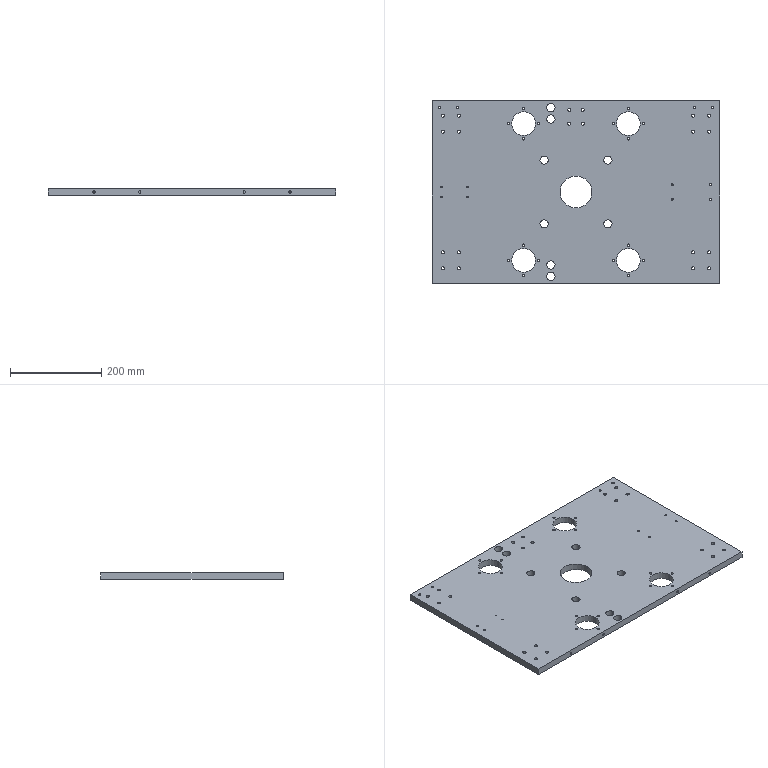Part | STEP file | 44-02-17 Press Cylinder Mounting Plate | 1 solid | 144 faces | box 630 x 400 x 15 mm | volume 3544491 mm3 | cylinder 130 | cone 8 | plane 6 | commonest cylinder face diameters 5 x48 7 x32 18 x16 3.3 x8 4.2 x8 6.8 x8